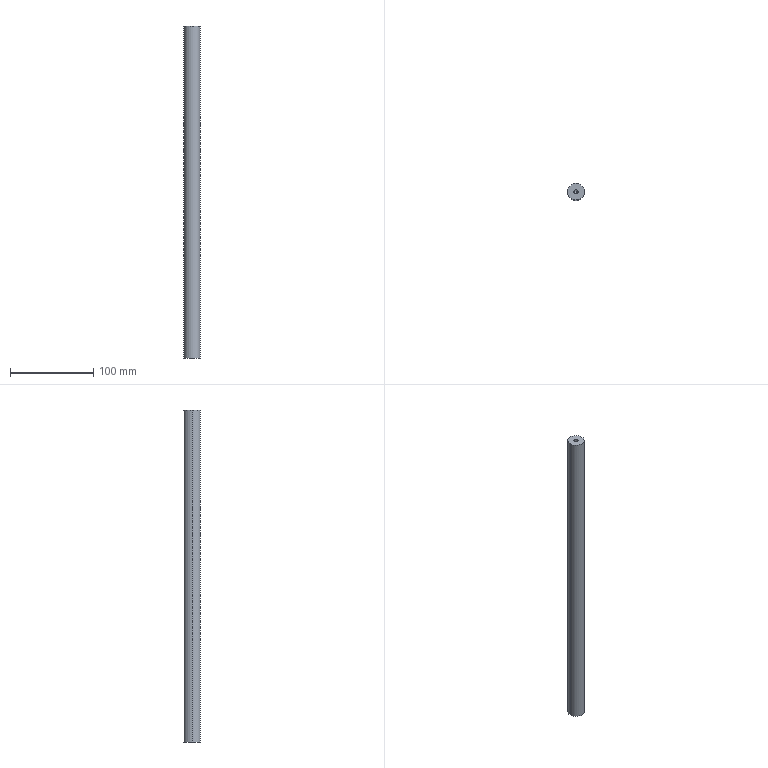Part | SolidWorks | features HoleWzd 2, Extrusion 1 | 1 solid | 12 faces | box 20 x 20 x 400 mm | volume 125055 mm3 | cylinder 6 | cone 4 | plane 2 | commonest cylinder face diameters 5 x4 20 x2
STEP:
#1=CARTESIAN_POINT('',(2.5,0.,15.));
#2=VERTEX_POINT('',#1);
#3=CARTESIAN_POINT('',(-2.5,0.,15.));
#4=VERTEX_POINT('',#3);
#5=CARTESIAN_POINT('',(0.,0.,15.));
#6=DIRECTION('',(0.,0.,-1.));
#7=DIRECTION('',(-1.,0.,0.));
#8=AXIS2_PLACEMENT_3D('',#5,#6,#7);
#9=CIRCLE('',#8,2.5);
#10=EDGE_CURVE('',#2,#4,#9,.T.);
#11=ORIENTED_EDGE('',*,*,#10,.F.);
#12=CARTESIAN_POINT('',(2.5,0.,0.));
#13=VERTEX_POINT('',#12);
#14=CARTESIAN_POINT('',(2.5,0.,0.));
#15=DIRECTION('',(0.,0.,-1.));
#16=VECTOR('',#15,1000.);
#17=LINE('',#14,#16);
#18=EDGE_CURVE('',#2,#13,#17,.T.);
#19=ORIENTED_EDGE('',*,*,#18,.T.);
#20=CARTESIAN_POINT('',(-2.5,0.,0.));
#21=VERTEX_POINT('',#20);
#22=CARTESIAN_POINT('',(0.,0.,0.));
#23=DIRECTION('',(0.,0.,-1.));
#24=DIRECTION('',(-1.,0.,0.));
#25=AXIS2_PLACEMENT_3D('',#22,#23,#24);
#26=CIRCLE('',#25,2.5);
#27=EDGE_CURVE('',#13,#21,#26,.T.);
#28=ORIENTED_EDGE('',*,*,#27,.T.);
#29=CARTESIAN_POINT('',(-2.5,0.,0.));
#30=DIRECTION('',(0.,0.,-1.));
#31=VECTOR('',#30,1000.);
#32=LINE('',#29,#31);
#33=EDGE_CURVE('',#4,#21,#32,.T.);
#34=ORIENTED_EDGE('',*,*,#33,.F.);
#35=EDGE_LOOP('',(#11,#19,#28,#34));
#36=FACE_OUTER_BOUND('',#35,.T.);
#37=CARTESIAN_POINT('',(0.,0.,0.));
#38=DIRECTION('',(0.,0.,-1.));
#39=DIRECTION('',(-1.,0.,0.));
#40=AXIS2_PLACEMENT_3D('',#37,#38,#39);
#41=CYLINDRICAL_SURFACE('',#40,2.5);
#42=ADVANCED_FACE('',(#36),#41,.F.);
#43=CARTESIAN_POINT('',(0.,0.,16.502));
#44=VERTEX_POINT('',#43);
#45=CARTESIAN_POINT('',(-2.5,0.,15.));
#46=DIRECTION('',(-0.8572,0.,-0.515));
#47=VECTOR('',#46,1000.);
#48=LINE('',#45,#47);
#49=EDGE_CURVE('',#44,#4,#48,.T.);
#50=ORIENTED_EDGE('',*,*,#49,.F.);
#51=CARTESIAN_POINT('',(2.5,0.,15.));
#52=DIRECTION('',(0.8572,0.,-0.515));
#53=VECTOR('',#52,1000.);
#54=LINE('',#51,#53);
#55=EDGE_CURVE('',#44,#2,#54,.T.);
#56=ORIENTED_EDGE('',*,*,#55,.T.);
#57=ORIENTED_EDGE('',*,*,#10,.T.);
#58=EDGE_LOOP('',(#50,#56,#57));
#59=FACE_OUTER_BOUND('',#58,.T.);
#60=CARTESIAN_POINT('',(0.,0.,15.));
#61=DIRECTION('',(0.,0.,-1.));
#62=DIRECTION('',(-1.,0.,0.));
#63=AXIS2_PLACEMENT_3D('',#60,#61,#62);
#64=CONICAL_SURFACE('',#63,2.5,1.03);
#65=ADVANCED_FACE('',(#59),#64,.F.);
#66=CARTESIAN_POINT('',(-2.5,0.,385.));
#67=VERTEX_POINT('',#66);
#68=CARTESIAN_POINT('',(2.5,0.,385.));
#69=VERTEX_POINT('',#68);
#70=CARTESIAN_POINT('',(0.,0.,385.));
#71=DIRECTION('',(0.,0.,1.));
#72=DIRECTION('',(1.,0.,0.));
#73=AXIS2_PLACEMENT_3D('',#70,#71,#72);
#74=CIRCLE('',#73,2.5);
#75=EDGE_CURVE('',#67,#69,#74,.T.);
#76=ORIENTED_EDGE('',*,*,#75,.F.);
#77=CARTESIAN_POINT('',(-2.5,0.,400.));
#78=VERTEX_POINT('',#77);
#79=CARTESIAN_POINT('',(-2.5,0.,400.));
#80=DIRECTION('',(0.,0.,1.));
#81=VECTOR('',#80,1000.);
#82=LINE('',#79,#81);
#83=EDGE_CURVE('',#67,#78,#82,.T.);
#84=ORIENTED_EDGE('',*,*,#83,.T.);
#85=CARTESIAN_POINT('',(2.5,0.,400.));
#86=VERTEX_POINT('',#85);
#87=CARTESIAN_POINT('',(0.,0.,400.));
#88=DIRECTION('',(0.,0.,1.));
#89=DIRECTION('',(1.,0.,0.));
#90=AXIS2_PLACEMENT_3D('',#87,#88,#89);
#91=CIRCLE('',#90,2.5);
#92=EDGE_CURVE('',#78,#86,#91,.T.);
#93=ORIENTED_EDGE('',*,*,#92,.T.);
#94=CARTESIAN_POINT('',(2.5,0.,400.));
#95=DIRECTION('',(0.,0.,1.));
#96=VECTOR('',#95,1000.);
#97=LINE('',#94,#96);
#98=EDGE_CURVE('',#69,#86,#97,.T.);
#99=ORIENTED_EDGE('',*,*,#98,.F.);
#100=EDGE_LOOP('',(#76,#84,#93,#99));
#101=FACE_OUTER_BOUND('',#100,.T.);
#102=CARTESIAN_POINT('',(0.,0.,400.));
#103=DIRECTION('',(0.,0.,1.));
#104=DIRECTION('',(1.,0.,0.));
#105=AXIS2_PLACEMENT_3D('',#102,#103,#104);
#106=CYLINDRICAL_SURFACE('',#105,2.5);
#107=ADVANCED_FACE('',(#101),#106,.F.);
#108=CARTESIAN_POINT('',(0.,0.,383.498));
#109=VERTEX_POINT('',#108);
#110=CARTESIAN_POINT('',(2.5,0.,385.));
#111=DIRECTION('',(0.8572,0.,0.515));
#112=VECTOR('',#111,1000.);
#113=LINE('',#110,#112);
#114=EDGE_CURVE('',#109,#69,#113,.T.);
#115=ORIENTED_EDGE('',*,*,#114,.F.);
#116=CARTESIAN_POINT('',(-2.5,0.,385.));
#117=DIRECTION('',(-0.8572,0.,0.515));
#118=VECTOR('',#117,1000.);
#119=LINE('',#116,#118);
#120=EDGE_CURVE('',#109,#67,#119,.T.);
#121=ORIENTED_EDGE('',*,*,#120,.T.);
#122=ORIENTED_EDGE('',*,*,#75,.T.);
#123=EDGE_LOOP('',(#115,#121,#122));
#124=FACE_OUTER_BOUND('',#123,.T.);
#125=CARTESIAN_POINT('',(0.,0.,385.));
#126=DIRECTION('',(0.,0.,1.));
#127=DIRECTION('',(1.,0.,0.));
#128=AXIS2_PLACEMENT_3D('',#125,#126,#127);
#129=CONICAL_SURFACE('',#128,2.5,1.03);
#130=ADVANCED_FACE('',(#124),#129,.F.);
#131=CARTESIAN_POINT('',(10.,0.,400.));
#132=VERTEX_POINT('',#131);
#133=CARTESIAN_POINT('',(-10.,0.,400.));
#134=VERTEX_POINT('',#133);
#135=CARTESIAN_POINT('',(0.,0.,400.));
#136=DIRECTION('',(0.,0.,1.));
#137=DIRECTION('',(1.,0.,0.));
#138=AXIS2_PLACEMENT_3D('',#135,#136,#137);
#139=CIRCLE('',#138,10.);
#140=EDGE_CURVE('',#132,#134,#139,.T.);
#141=ORIENTED_EDGE('',*,*,#140,.F.);
#142=CARTESIAN_POINT('',(10.,0.,0.));
#143=VERTEX_POINT('',#142);
#144=CARTESIAN_POINT('',(10.,0.,400.));
#145=DIRECTION('',(0.,0.,-1.));
#146=VECTOR('',#145,1000.);
#147=LINE('',#144,#146);
#148=EDGE_CURVE('',#132,#143,#147,.T.);
#149=ORIENTED_EDGE('',*,*,#148,.T.);
#150=CARTESIAN_POINT('',(-10.,0.,0.));
#151=VERTEX_POINT('',#150);
#152=CARTESIAN_POINT('',(0.,0.,0.));
#153=DIRECTION('',(0.,0.,1.));
#154=DIRECTION('',(1.,0.,0.));
#155=AXIS2_PLACEMENT_3D('',#152,#153,#154);
#156=CIRCLE('',#155,10.);
#157=EDGE_CURVE('',#143,#151,#156,.T.);
#158=ORIENTED_EDGE('',*,*,#157,.T.);
#159=CARTESIAN_POINT('',(-10.,0.,400.));
#160=DIRECTION('',(0.,0.,-1.));
#161=VECTOR('',#160,1000.);
#162=LINE('',#159,#161);
#163=EDGE_CURVE('',#134,#151,#162,.T.);
#164=ORIENTED_EDGE('',*,*,#163,.F.);
#165=EDGE_LOOP('',(#141,#149,#158,#164));
#166=FACE_OUTER_BOUND('',#165,.T.);
#167=CARTESIAN_POINT('',(0.,0.,400.));
#168=DIRECTION('',(0.,0.,-1.));
#169=DIRECTION('',(-1.,0.,0.));
#170=AXIS2_PLACEMENT_3D('',#167,#168,#169);
#171=CYLINDRICAL_SURFACE('',#170,10.);
#172=ADVANCED_FACE('',(#166),#171,.T.);
#173=ORIENTED_EDGE('',*,*,#148,.F.);
#174=CARTESIAN_POINT('',(0.,0.,400.));
#175=DIRECTION('',(0.,0.,1.));
#176=DIRECTION('',(1.,0.,0.));
#177=AXIS2_PLACEMENT_3D('',#174,#175,#176);
#178=CIRCLE('',#177,10.);
#179=EDGE_CURVE('',#134,#132,#178,.T.);
#180=ORIENTED_EDGE('',*,*,#179,.F.);
#181=ORIENTED_EDGE('',*,*,#163,.T.);
#182=CARTESIAN_POINT('',(0.,0.,0.));
#183=DIRECTION('',(0.,0.,1.));
#184=DIRECTION('',(1.,0.,0.));
#185=AXIS2_PLACEMENT_3D('',#182,#183,#184);
#186=CIRCLE('',#185,10.);
#187=EDGE_CURVE('',#151,#143,#186,.T.);
#188=ORIENTED_EDGE('',*,*,#187,.T.);
#189=EDGE_LOOP('',(#173,#180,#181,#188));
#190=FACE_OUTER_BOUND('',#189,.T.);
#191=CARTESIAN_POINT('',(0.,0.,400.));
#192=DIRECTION('',(0.,0.,-1.));
#193=DIRECTION('',(-1.,0.,0.));
#194=AXIS2_PLACEMENT_3D('',#191,#192,#193);
#195=CYLINDRICAL_SURFACE('',#194,10.);
#196=ADVANCED_FACE('',(#190),#195,.T.);
#197=CARTESIAN_POINT('',(0.,0.,400.));
#198=DIRECTION('',(0.,0.,1.));
#199=DIRECTION('',(1.,0.,0.));
#200=AXIS2_PLACEMENT_3D('',#197,#198,#199);
#201=CIRCLE('',#200,2.5);
#202=EDGE_CURVE('',#86,#78,#201,.T.);
#203=ORIENTED_EDGE('',*,*,#202,.F.);
#204=ORIENTED_EDGE('',*,*,#92,.F.);
#205=EDGE_LOOP('',(#203,#204));
#206=FACE_BOUND('',#205,.T.);
#207=ORIENTED_EDGE('',*,*,#179,.T.);
#208=ORIENTED_EDGE('',*,*,#140,.T.);
#209=EDGE_LOOP('',(#207,#208));
#210=FACE_OUTER_BOUND('',#209,.T.);
#211=CARTESIAN_POINT('',(0.,0.,400.));
#212=DIRECTION('',(0.,0.,1.));
#213=DIRECTION('',(1.,0.,0.));
#214=AXIS2_PLACEMENT_3D('',#211,#212,#213);
#215=PLANE('',#214);
#216=ADVANCED_FACE('',(#206,#210),#215,.T.);
#217=CARTESIAN_POINT('',(0.,0.,0.));
#218=DIRECTION('',(0.,0.,-1.));
#219=DIRECTION('',(-1.,0.,0.));
#220=AXIS2_PLACEMENT_3D('',#217,#218,#219);
#221=CIRCLE('',#220,2.5);
#222=EDGE_CURVE('',#21,#13,#221,.T.);
#223=ORIENTED_EDGE('',*,*,#222,.F.);
#224=ORIENTED_EDGE('',*,*,#27,.F.);
#225=EDGE_LOOP('',(#223,#224));
#226=FACE_BOUND('',#225,.T.);
#227=ORIENTED_EDGE('',*,*,#187,.F.);
#228=ORIENTED_EDGE('',*,*,#157,.F.);
#229=EDGE_LOOP('',(#227,#228));
#230=FACE_OUTER_BOUND('',#229,.T.);
#231=CARTESIAN_POINT('',(0.,0.,0.));
#232=DIRECTION('',(0.,0.,1.));
#233=DIRECTION('',(1.,0.,0.));
#234=AXIS2_PLACEMENT_3D('',#231,#232,#233);
#235=PLANE('',#234);
#236=ADVANCED_FACE('',(#226,#230),#235,.F.);
#237=ORIENTED_EDGE('',*,*,#120,.F.);
#238=ORIENTED_EDGE('',*,*,#114,.T.);
#239=CARTESIAN_POINT('',(0.,0.,385.));
#240=DIRECTION('',(0.,0.,1.));
#241=DIRECTION('',(1.,0.,0.));
#242=AXIS2_PLACEMENT_3D('',#239,#240,#241);
#243=CIRCLE('',#242,2.5);
#244=EDGE_CURVE('',#69,#67,#243,.T.);
#245=ORIENTED_EDGE('',*,*,#244,.T.);
#246=EDGE_LOOP('',(#237,#238,#245));
#247=FACE_OUTER_BOUND('',#246,.T.);
#248=CARTESIAN_POINT('',(0.,0.,385.));
#249=DIRECTION('',(0.,0.,1.));
#250=DIRECTION('',(1.,0.,0.));
#251=AXIS2_PLACEMENT_3D('',#248,#249,#250);
#252=CONICAL_SURFACE('',#251,2.5,1.03);
#253=ADVANCED_FACE('',(#247),#252,.F.);
#254=ORIENTED_EDGE('',*,*,#83,.F.);
#255=ORIENTED_EDGE('',*,*,#244,.F.);
#256=ORIENTED_EDGE('',*,*,#98,.T.);
#257=ORIENTED_EDGE('',*,*,#202,.T.);
#258=EDGE_LOOP('',(#254,#255,#256,#257));
#259=FACE_OUTER_BOUND('',#258,.T.);
#260=CARTESIAN_POINT('',(0.,0.,400.));
#261=DIRECTION('',(0.,0.,1.));
#262=DIRECTION('',(1.,0.,0.));
#263=AXIS2_PLACEMENT_3D('',#260,#261,#262);
#264=CYLINDRICAL_SURFACE('',#263,2.5);
#265=ADVANCED_FACE('',(#259),#264,.F.);
#266=ORIENTED_EDGE('',*,*,#55,.F.);
#267=ORIENTED_EDGE('',*,*,#49,.T.);
#268=CARTESIAN_POINT('',(0.,0.,15.));
#269=DIRECTION('',(0.,0.,-1.));
#270=DIRECTION('',(-1.,0.,0.));
#271=AXIS2_PLACEMENT_3D('',#268,#269,#270);
#272=CIRCLE('',#271,2.5);
#273=EDGE_CURVE('',#4,#2,#272,.T.);
#274=ORIENTED_EDGE('',*,*,#273,.T.);
#275=EDGE_LOOP('',(#266,#267,#274));
#276=FACE_OUTER_BOUND('',#275,.T.);
#277=CARTESIAN_POINT('',(0.,0.,15.));
#278=DIRECTION('',(0.,0.,-1.));
#279=DIRECTION('',(-1.,0.,0.));
#280=AXIS2_PLACEMENT_3D('',#277,#278,#279);
#281=CONICAL_SURFACE('',#280,2.5,1.03);
#282=ADVANCED_FACE('',(#276),#281,.F.);
#283=ORIENTED_EDGE('',*,*,#18,.F.);
#284=ORIENTED_EDGE('',*,*,#273,.F.);
#285=ORIENTED_EDGE('',*,*,#33,.T.);
#286=ORIENTED_EDGE('',*,*,#222,.T.);
#287=EDGE_LOOP('',(#283,#284,#285,#286));
#288=FACE_OUTER_BOUND('',#287,.T.);
#289=CARTESIAN_POINT('',(0.,0.,0.));
#290=DIRECTION('',(0.,0.,-1.));
#291=DIRECTION('',(-1.,0.,0.));
#292=AXIS2_PLACEMENT_3D('',#289,#290,#291);
#293=CYLINDRICAL_SURFACE('',#292,2.5);
#294=ADVANCED_FACE('',(#288),#293,.F.);
#295=CLOSED_SHELL('',(#42,#65,#107,#130,#172,#196,#216,#236,#253,#265,#282,#294));
#296=MANIFOLD_SOLID_BREP('',#295);
#297=CARTESIAN_POINT('',(0.,0.,0.));
#298=DIRECTION('',(0.,0.,1.));
#299=DIRECTION('',(1.,0.,0.));
#300=AXIS2_PLACEMENT_3D('',#297,#298,#299);
#301=(LENGTH_UNIT()NAMED_UNIT(*)SI_UNIT(.MILLI.,.METRE.));
#302=UNCERTAINTY_MEASURE_WITH_UNIT(LENGTH_MEASURE(0.00001),#301,'','');
#303=(NAMED_UNIT(*)PLANE_ANGLE_UNIT()SI_UNIT($,.RADIAN.));
#304=(NAMED_UNIT(*)SI_UNIT($,.STERADIAN.)SOLID_ANGLE_UNIT());
#305=(GEOMETRIC_REPRESENTATION_CONTEXT(3)GLOBAL_UNCERTAINTY_ASSIGNED_CONTEXT((#302))GLOBAL_UNIT_ASSIGNED_CONTEXT((#301,#303,#304))REPRESENTATION_CONTEXT('',''));
#306=ADVANCED_BREP_SHAPE_REPRESENTATION('',(#296,#300),#305);